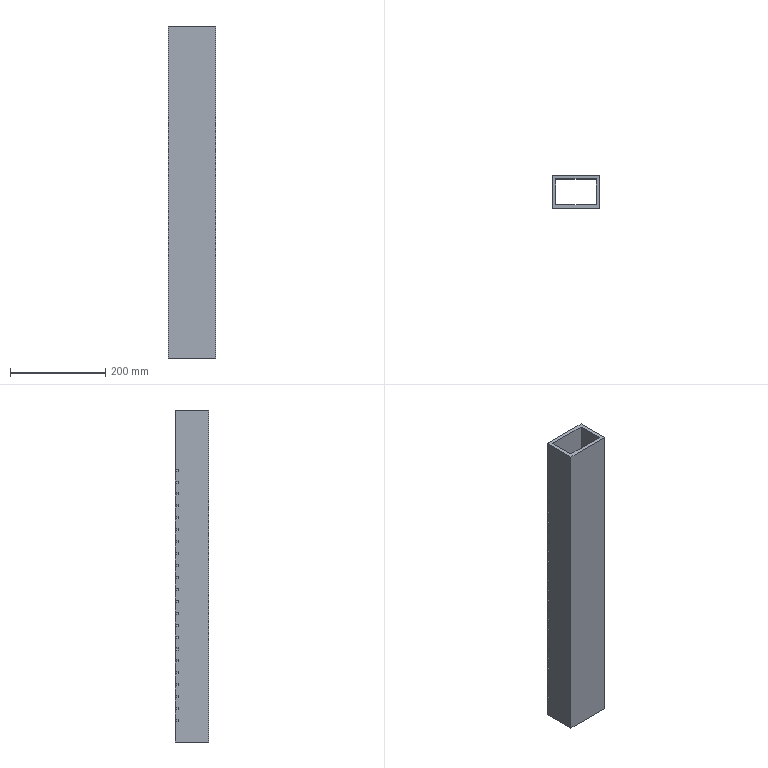Part | SolidWorks | features BaseBody 1 | 1 solid | 118 faces | box 100 x 70 x 696 mm | volume 1711198 mm3 | cylinder 64 | plane 54 | commonest cylinder face diameters 4.3 x44 5.3 x20